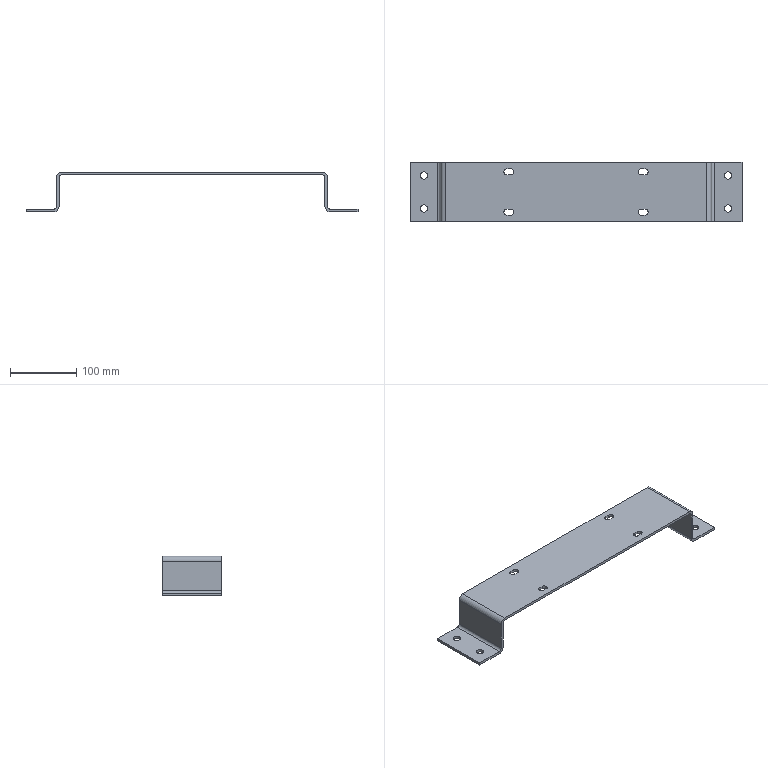Part | STEP file | HL4GZ-1.581.108 (auxiliary valve bracket) | 1 solid | 42 faces | box 502 x 90 x 60 mm | volume 213929 mm3 | plane 22 | cylinder 20 | commonest cylinder face diameters 9 x8 8 x4 11 x4 16 x4